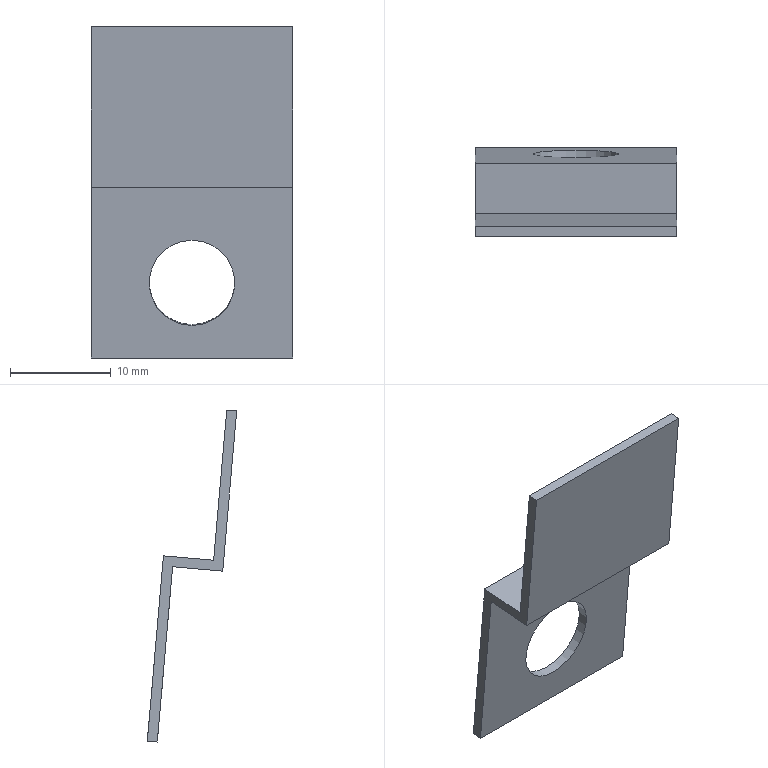Part | NX | features solid 2 | 1 solid | 11 faces | box 20 x 8.897 x 33.024 mm | volume 713.255 mm3 | plane 10 | cylinder 1 | commonest cylinder face diameters 8.5 x1
STEP:
#1=CARTESIAN_POINT('',(-140.187,114.602,-61.476));
#2=VERTEX_POINT('',#1);
#3=CARTESIAN_POINT('',(-160.187,114.602,-61.476));
#4=VERTEX_POINT('',#3);
#5=CARTESIAN_POINT('',(-140.187,114.602,-61.476));
#6=DIRECTION('',(-1.,0.,0.));
#7=VECTOR('',#6,1000.);
#8=LINE('',#5,#7);
#9=EDGE_CURVE('',#2,#4,#8,.T.);
#10=ORIENTED_EDGE('',*,*,#9,.F.);
#11=CARTESIAN_POINT('',(-140.187,116.214,-79.905));
#12=VERTEX_POINT('',#11);
#13=CARTESIAN_POINT('',(-140.187,114.689,-62.472));
#14=DIRECTION('',(0.,-0.08716,0.9962));
#15=VECTOR('',#14,1000.);
#16=LINE('',#13,#15);
#17=EDGE_CURVE('',#12,#2,#16,.T.);
#18=ORIENTED_EDGE('',*,*,#17,.F.);
#19=CARTESIAN_POINT('',(-160.187,116.214,-79.905));
#20=VERTEX_POINT('',#19);
#21=CARTESIAN_POINT('',(-140.187,116.214,-79.905));
#22=DIRECTION('',(-1.,0.,0.));
#23=VECTOR('',#22,1000.);
#24=LINE('',#21,#23);
#25=EDGE_CURVE('',#12,#20,#24,.T.);
#26=ORIENTED_EDGE('',*,*,#25,.T.);
#27=CARTESIAN_POINT('',(-160.187,114.602,-61.476));
#28=DIRECTION('',(0.,0.08716,-0.9962));
#29=VECTOR('',#28,1000.);
#30=LINE('',#27,#29);
#31=EDGE_CURVE('',#4,#20,#30,.T.);
#32=ORIENTED_EDGE('',*,*,#31,.F.);
#33=EDGE_LOOP('',(#10,#18,#26,#32));
#34=FACE_BOUND('',#33,.T.);
#35=CARTESIAN_POINT('',(-150.187,115.931,-76.668));
#36=VERTEX_POINT('',#35);
#37=CARTESIAN_POINT('',(-150.187,115.561,-72.434));
#38=DIRECTION('',(0.,-0.9962,-0.08716));
#39=DIRECTION('',(0.,0.08716,-0.9962));
#40=AXIS2_PLACEMENT_3D('',#37,#38,#39);
#41=CIRCLE('',#40,4.25);
#42=EDGE_CURVE('',#36,#36,#41,.T.);
#43=ORIENTED_EDGE('',*,*,#42,.T.);
#44=EDGE_LOOP('',(#43));
#45=FACE_BOUND('',#44,.T.);
#46=CARTESIAN_POINT('',(-160.187,114.602,-61.476));
#47=DIRECTION('',(0.,-0.9962,-0.08716));
#48=DIRECTION('',(0.,0.08716,-0.9962));
#49=AXIS2_PLACEMENT_3D('',#46,#47,#48);
#50=PLANE('',#49);
#51=ADVANCED_FACE('',(#34,#45),#50,.F.);
#52=CARTESIAN_POINT('',(-140.187,115.218,-79.992));
#53=VERTEX_POINT('',#52);
#54=CARTESIAN_POINT('',(-160.187,115.218,-79.992));
#55=VERTEX_POINT('',#54);
#56=CARTESIAN_POINT('',(-140.187,115.218,-79.992));
#57=DIRECTION('',(-1.,0.,0.));
#58=VECTOR('',#57,1000.);
#59=LINE('',#56,#58);
#60=EDGE_CURVE('',#53,#55,#59,.T.);
#61=ORIENTED_EDGE('',*,*,#60,.F.);
#62=CARTESIAN_POINT('',(-140.187,113.693,-62.559));
#63=VERTEX_POINT('',#62);
#64=CARTESIAN_POINT('',(-140.187,113.693,-62.559));
#65=DIRECTION('',(0.,0.08716,-0.9962));
#66=VECTOR('',#65,1000.);
#67=LINE('',#64,#66);
#68=EDGE_CURVE('',#63,#53,#67,.T.);
#69=ORIENTED_EDGE('',*,*,#68,.F.);
#70=CARTESIAN_POINT('',(-160.187,113.693,-62.559));
#71=VERTEX_POINT('',#70);
#72=CARTESIAN_POINT('',(-140.187,113.693,-62.559));
#73=DIRECTION('',(-1.,0.,0.));
#74=VECTOR('',#73,1000.);
#75=LINE('',#72,#74);
#76=EDGE_CURVE('',#63,#71,#75,.T.);
#77=ORIENTED_EDGE('',*,*,#76,.T.);
#78=CARTESIAN_POINT('',(-160.187,115.218,-79.992));
#79=DIRECTION('',(0.,-0.08716,0.9962));
#80=VECTOR('',#79,1000.);
#81=LINE('',#78,#80);
#82=EDGE_CURVE('',#55,#71,#81,.T.);
#83=ORIENTED_EDGE('',*,*,#82,.F.);
#84=EDGE_LOOP('',(#61,#69,#77,#83));
#85=FACE_BOUND('',#84,.T.);
#86=CARTESIAN_POINT('',(-150.187,114.935,-76.755));
#87=VERTEX_POINT('',#86);
#88=CARTESIAN_POINT('',(-150.187,114.564,-72.521));
#89=DIRECTION('',(0.,-0.9962,-0.08716));
#90=DIRECTION('',(0.,0.08716,-0.9962));
#91=AXIS2_PLACEMENT_3D('',#88,#89,#90);
#92=CIRCLE('',#91,4.25);
#93=EDGE_CURVE('',#87,#87,#92,.T.);
#94=ORIENTED_EDGE('',*,*,#93,.F.);
#95=EDGE_LOOP('',(#94));
#96=FACE_BOUND('',#95,.T.);
#97=CARTESIAN_POINT('',(-160.187,115.218,-79.992));
#98=DIRECTION('',(0.,0.9962,0.08716));
#99=DIRECTION('',(0.,-0.08716,0.9962));
#100=AXIS2_PLACEMENT_3D('',#97,#98,#99);
#101=PLANE('',#100);
#102=ADVANCED_FACE('',(#85,#96),#101,.F.);
#103=CARTESIAN_POINT('',(-160.187,108.314,-46.969));
#104=VERTEX_POINT('',#103);
#105=CARTESIAN_POINT('',(-140.187,108.314,-46.969));
#106=VERTEX_POINT('',#105);
#107=CARTESIAN_POINT('',(-160.187,108.314,-46.969));
#108=DIRECTION('',(1.,0.,0.));
#109=VECTOR('',#108,1000.);
#110=LINE('',#107,#109);
#111=EDGE_CURVE('',#104,#106,#110,.T.);
#112=ORIENTED_EDGE('',*,*,#111,.F.);
#113=CARTESIAN_POINT('',(-160.187,107.317,-47.056));
#114=VERTEX_POINT('',#113);
#115=CARTESIAN_POINT('',(-160.187,107.317,-47.056));
#116=DIRECTION('',(0.,0.9962,0.08716));
#117=VECTOR('',#116,1000.);
#118=LINE('',#115,#117);
#119=EDGE_CURVE('',#114,#104,#118,.T.);
#120=ORIENTED_EDGE('',*,*,#119,.F.);
#121=CARTESIAN_POINT('',(-140.187,107.317,-47.056));
#122=VERTEX_POINT('',#121);
#123=CARTESIAN_POINT('',(-160.187,107.317,-47.056));
#124=DIRECTION('',(1.,0.,0.));
#125=VECTOR('',#124,1000.);
#126=LINE('',#123,#125);
#127=EDGE_CURVE('',#114,#122,#126,.T.);
#128=ORIENTED_EDGE('',*,*,#127,.T.);
#129=CARTESIAN_POINT('',(-140.187,107.317,-47.056));
#130=DIRECTION('',(0.,0.9962,0.08716));
#131=VECTOR('',#130,1000.);
#132=LINE('',#129,#131);
#133=EDGE_CURVE('',#122,#106,#132,.T.);
#134=ORIENTED_EDGE('',*,*,#133,.T.);
#135=EDGE_LOOP('',(#112,#120,#128,#134));
#136=FACE_BOUND('',#135,.T.);
#137=CARTESIAN_POINT('',(-160.187,107.317,-47.056));
#138=DIRECTION('',(0.,-0.08716,0.9962));
#139=DIRECTION('',(0.,-0.9962,-0.08716));
#140=AXIS2_PLACEMENT_3D('',#137,#138,#139);
#141=PLANE('',#140);
#142=ADVANCED_FACE('',(#136),#141,.T.);
#143=CARTESIAN_POINT('',(-140.187,109.621,-61.912));
#144=VERTEX_POINT('',#143);
#145=CARTESIAN_POINT('',(-140.187,108.314,-46.969));
#146=DIRECTION('',(0.,0.08716,-0.9962));
#147=VECTOR('',#146,1000.);
#148=LINE('',#145,#147);
#149=EDGE_CURVE('',#106,#144,#148,.T.);
#150=ORIENTED_EDGE('',*,*,#149,.F.);
#151=ORIENTED_EDGE('',*,*,#133,.F.);
#152=CARTESIAN_POINT('',(-140.187,108.712,-62.995));
#153=VERTEX_POINT('',#152);
#154=CARTESIAN_POINT('',(-140.187,107.317,-47.056));
#155=DIRECTION('',(0.,0.08716,-0.9962));
#156=VECTOR('',#155,1000.);
#157=LINE('',#154,#156);
#158=EDGE_CURVE('',#122,#153,#157,.T.);
#159=ORIENTED_EDGE('',*,*,#158,.T.);
#160=CARTESIAN_POINT('',(-140.187,108.712,-62.995));
#161=DIRECTION('',(0.,0.9962,0.08716));
#162=VECTOR('',#161,1000.);
#163=LINE('',#160,#162);
#164=EDGE_CURVE('',#153,#63,#163,.T.);
#165=ORIENTED_EDGE('',*,*,#164,.T.);
#166=ORIENTED_EDGE('',*,*,#68,.T.);
#167=CARTESIAN_POINT('',(-140.187,115.218,-79.992));
#168=DIRECTION('',(0.,0.9962,0.08716));
#169=VECTOR('',#168,1000.);
#170=LINE('',#167,#169);
#171=EDGE_CURVE('',#53,#12,#170,.T.);
#172=ORIENTED_EDGE('',*,*,#171,.T.);
#173=ORIENTED_EDGE('',*,*,#17,.T.);
#174=CARTESIAN_POINT('',(-140.187,108.625,-61.999));
#175=DIRECTION('',(0.,0.9962,0.08716));
#176=VECTOR('',#175,1000.);
#177=LINE('',#174,#176);
#178=EDGE_CURVE('',#144,#2,#177,.T.);
#179=ORIENTED_EDGE('',*,*,#178,.F.);
#180=EDGE_LOOP('',(#150,#151,#159,#165,#166,#172,#173,#179));
#181=FACE_BOUND('',#180,.T.);
#182=CARTESIAN_POINT('',(-140.187,107.317,-47.056));
#183=DIRECTION('',(1.,0.,0.));
#184=DIRECTION('',(0.,-0.9962,-0.08716));
#185=AXIS2_PLACEMENT_3D('',#182,#183,#184);
#186=PLANE('',#185);
#187=ADVANCED_FACE('',(#181),#186,.T.);
#188=CARTESIAN_POINT('',(-160.187,109.621,-61.912));
#189=VERTEX_POINT('',#188);
#190=CARTESIAN_POINT('',(-160.187,109.621,-61.912));
#191=DIRECTION('',(0.,-0.08716,0.9962));
#192=VECTOR('',#191,1000.);
#193=LINE('',#190,#192);
#194=EDGE_CURVE('',#189,#104,#193,.T.);
#195=ORIENTED_EDGE('',*,*,#194,.F.);
#196=CARTESIAN_POINT('',(-160.187,108.625,-61.999));
#197=DIRECTION('',(0.,0.9962,0.08716));
#198=VECTOR('',#197,1000.);
#199=LINE('',#196,#198);
#200=EDGE_CURVE('',#189,#4,#199,.T.);
#201=ORIENTED_EDGE('',*,*,#200,.T.);
#202=ORIENTED_EDGE('',*,*,#31,.T.);
#203=CARTESIAN_POINT('',(-160.187,115.218,-79.992));
#204=DIRECTION('',(0.,0.9962,0.08716));
#205=VECTOR('',#204,1000.);
#206=LINE('',#203,#205);
#207=EDGE_CURVE('',#55,#20,#206,.T.);
#208=ORIENTED_EDGE('',*,*,#207,.F.);
#209=ORIENTED_EDGE('',*,*,#82,.T.);
#210=CARTESIAN_POINT('',(-160.187,108.712,-62.995));
#211=VERTEX_POINT('',#210);
#212=CARTESIAN_POINT('',(-160.187,108.712,-62.995));
#213=DIRECTION('',(0.,0.9962,0.08716));
#214=VECTOR('',#213,1000.);
#215=LINE('',#212,#214);
#216=EDGE_CURVE('',#211,#71,#215,.T.);
#217=ORIENTED_EDGE('',*,*,#216,.F.);
#218=CARTESIAN_POINT('',(-160.187,108.625,-61.999));
#219=DIRECTION('',(0.,-0.08716,0.9962));
#220=VECTOR('',#219,1000.);
#221=LINE('',#218,#220);
#222=EDGE_CURVE('',#211,#114,#221,.T.);
#223=ORIENTED_EDGE('',*,*,#222,.T.);
#224=ORIENTED_EDGE('',*,*,#119,.T.);
#225=EDGE_LOOP('',(#195,#201,#202,#208,#209,#217,#223,#224));
#226=FACE_BOUND('',#225,.T.);
#227=CARTESIAN_POINT('',(-160.187,108.625,-61.999));
#228=DIRECTION('',(-1.,0.,0.));
#229=DIRECTION('',(0.,0.08716,-0.9962));
#230=AXIS2_PLACEMENT_3D('',#227,#228,#229);
#231=PLANE('',#230);
#232=ADVANCED_FACE('',(#226),#231,.T.);
#233=ORIENTED_EDGE('',*,*,#127,.F.);
#234=ORIENTED_EDGE('',*,*,#222,.F.);
#235=CARTESIAN_POINT('',(-140.187,108.712,-62.995));
#236=DIRECTION('',(-1.,0.,0.));
#237=VECTOR('',#236,1000.);
#238=LINE('',#235,#237);
#239=EDGE_CURVE('',#153,#211,#238,.T.);
#240=ORIENTED_EDGE('',*,*,#239,.F.);
#241=ORIENTED_EDGE('',*,*,#158,.F.);
#242=EDGE_LOOP('',(#233,#234,#240,#241));
#243=FACE_BOUND('',#242,.T.);
#244=CARTESIAN_POINT('',(-140.187,107.317,-47.056));
#245=DIRECTION('',(0.,0.9962,0.08716));
#246=DIRECTION('',(0.,-0.08716,0.9962));
#247=AXIS2_PLACEMENT_3D('',#244,#245,#246);
#248=PLANE('',#247);
#249=ADVANCED_FACE('',(#243),#248,.F.);
#250=ORIENTED_EDGE('',*,*,#111,.T.);
#251=ORIENTED_EDGE('',*,*,#149,.T.);
#252=CARTESIAN_POINT('',(-140.187,109.621,-61.912));
#253=DIRECTION('',(-1.,0.,0.));
#254=VECTOR('',#253,1000.);
#255=LINE('',#252,#254);
#256=EDGE_CURVE('',#144,#189,#255,.T.);
#257=ORIENTED_EDGE('',*,*,#256,.T.);
#258=ORIENTED_EDGE('',*,*,#194,.T.);
#259=EDGE_LOOP('',(#250,#251,#257,#258));
#260=FACE_BOUND('',#259,.T.);
#261=CARTESIAN_POINT('',(-140.187,108.314,-46.969));
#262=DIRECTION('',(0.,0.9962,0.08716));
#263=DIRECTION('',(0.,-0.08716,0.9962));
#264=AXIS2_PLACEMENT_3D('',#261,#262,#263);
#265=PLANE('',#264);
#266=ADVANCED_FACE('',(#260),#265,.T.);
#267=ORIENTED_EDGE('',*,*,#256,.F.);
#268=ORIENTED_EDGE('',*,*,#178,.T.);
#269=ORIENTED_EDGE('',*,*,#9,.T.);
#270=ORIENTED_EDGE('',*,*,#200,.F.);
#271=EDGE_LOOP('',(#267,#268,#269,#270));
#272=FACE_BOUND('',#271,.T.);
#273=CARTESIAN_POINT('',(-140.187,108.625,-61.999));
#274=DIRECTION('',(0.,0.08716,-0.9962));
#275=DIRECTION('',(0.,0.9962,0.08716));
#276=AXIS2_PLACEMENT_3D('',#273,#274,#275);
#277=PLANE('',#276);
#278=ADVANCED_FACE('',(#272),#277,.F.);
#279=ORIENTED_EDGE('',*,*,#76,.F.);
#280=ORIENTED_EDGE('',*,*,#164,.F.);
#281=ORIENTED_EDGE('',*,*,#239,.T.);
#282=ORIENTED_EDGE('',*,*,#216,.T.);
#283=EDGE_LOOP('',(#279,#280,#281,#282));
#284=FACE_BOUND('',#283,.T.);
#285=CARTESIAN_POINT('',(-140.187,108.712,-62.995));
#286=DIRECTION('',(0.,0.08716,-0.9962));
#287=DIRECTION('',(0.,0.9962,0.08716));
#288=AXIS2_PLACEMENT_3D('',#285,#286,#287);
#289=PLANE('',#288);
#290=ADVANCED_FACE('',(#284),#289,.T.);
#291=ORIENTED_EDGE('',*,*,#25,.F.);
#292=ORIENTED_EDGE('',*,*,#171,.F.);
#293=ORIENTED_EDGE('',*,*,#60,.T.);
#294=ORIENTED_EDGE('',*,*,#207,.T.);
#295=EDGE_LOOP('',(#291,#292,#293,#294));
#296=FACE_BOUND('',#295,.T.);
#297=CARTESIAN_POINT('',(-140.187,115.218,-79.992));
#298=DIRECTION('',(0.,0.08716,-0.9962));
#299=DIRECTION('',(0.,0.9962,0.08716));
#300=AXIS2_PLACEMENT_3D('',#297,#298,#299);
#301=PLANE('',#300);
#302=ADVANCED_FACE('',(#296),#301,.T.);
#303=ORIENTED_EDGE('',*,*,#93,.T.);
#304=EDGE_LOOP('',(#303));
#305=FACE_BOUND('',#304,.T.);
#306=ORIENTED_EDGE('',*,*,#42,.F.);
#307=EDGE_LOOP('',(#306));
#308=FACE_BOUND('',#307,.T.);
#309=CARTESIAN_POINT('',(-150.187,114.564,-72.521));
#310=DIRECTION('',(0.,0.9962,0.08716));
#311=DIRECTION('',(0.,-0.08716,0.9962));
#312=AXIS2_PLACEMENT_3D('',#309,#310,#311);
#313=CYLINDRICAL_SURFACE('',#312,4.25);
#314=ADVANCED_FACE('',(#305,#308),#313,.F.);
#315=CLOSED_SHELL('',(#51,#102,#142,#187,#232,#249,#266,#278,#290,#302,#314));
#316=MANIFOLD_SOLID_BREP('',#315);
#317=(LENGTH_UNIT()NAMED_UNIT(*)SI_UNIT(.MILLI.,.METRE.));
#318=UNCERTAINTY_MEASURE_WITH_UNIT(LENGTH_MEASURE(0.00001),#317,'','');
#319=(NAMED_UNIT(*)PLANE_ANGLE_UNIT()SI_UNIT($,.RADIAN.));
#320=(NAMED_UNIT(*)SI_UNIT($,.STERADIAN.)SOLID_ANGLE_UNIT());
#321=(GEOMETRIC_REPRESENTATION_CONTEXT(3)GLOBAL_UNCERTAINTY_ASSIGNED_CONTEXT((#318))GLOBAL_UNIT_ASSIGNED_CONTEXT((#317,#319,#320))REPRESENTATION_CONTEXT('',''));
#322=ADVANCED_BREP_SHAPE_REPRESENTATION('',(#316),#321);